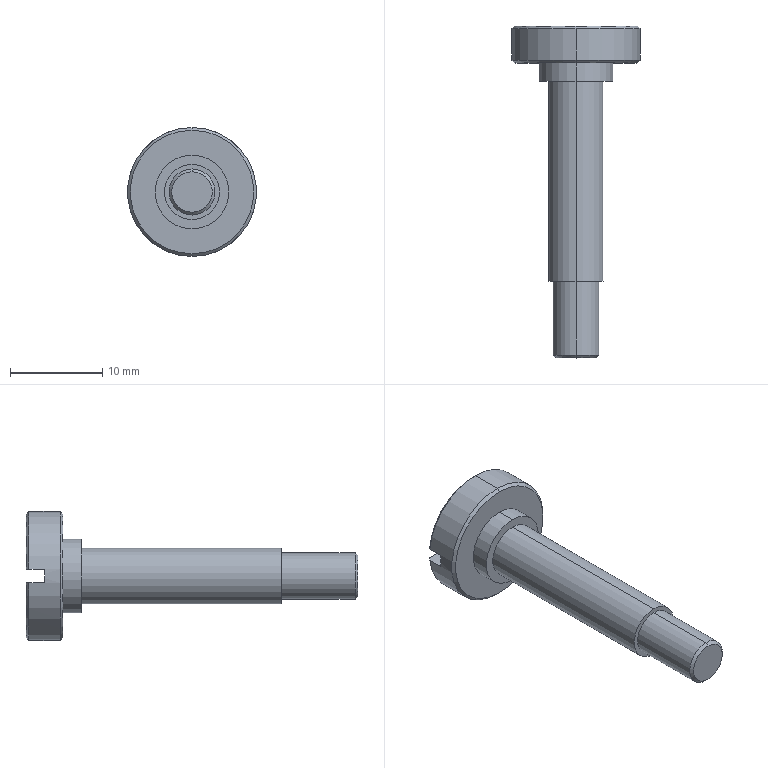Part | SolidWorks | features BaseBody 1 | 1 solid | 24 faces | box 14 x 36 x 14 mm | volume 1446 mm3 | plane 9 | cylinder 8 | cone 7 | commonest cylinder face diameters 5 x2 6 x2 8 x2 14 x2
STEP:
#1=CARTESIAN_POINT('',(0.,36.,-6.7));
#2=VERTEX_POINT('',#1);
#3=CARTESIAN_POINT('',(-6.658,36.,-0.75));
#4=VERTEX_POINT('',#3);
#5=CARTESIAN_POINT('',(0.,36.,0.));
#6=DIRECTION('',(0.,1.,0.));
#7=DIRECTION('',(0.,0.,-1.));
#8=AXIS2_PLACEMENT_3D('',#5,#6,#7);
#9=CIRCLE('',#8,6.7);
#10=EDGE_CURVE('',#2,#4,#9,.T.);
#11=ORIENTED_EDGE('',*,*,#10,.F.);
#12=CARTESIAN_POINT('',(0.,35.7,-7.));
#13=VERTEX_POINT('',#12);
#14=CARTESIAN_POINT('',(0.,35.7,-7.));
#15=DIRECTION('',(0.,-0.7071,-0.7071));
#16=VECTOR('',#15,1000.);
#17=LINE('',#14,#16);
#18=EDGE_CURVE('',#2,#13,#17,.T.);
#19=ORIENTED_EDGE('',*,*,#18,.T.);
#20=CARTESIAN_POINT('',(-6.96,35.7,-0.75));
#21=VERTEX_POINT('',#20);
#22=CARTESIAN_POINT('',(0.,35.7,0.));
#23=DIRECTION('',(0.,-1.,0.));
#24=DIRECTION('',(0.,0.,-1.));
#25=AXIS2_PLACEMENT_3D('',#22,#23,#24);
#26=CIRCLE('',#25,7.);
#27=EDGE_CURVE('',#21,#13,#26,.T.);
#28=ORIENTED_EDGE('',*,*,#27,.F.);
#29=CARTESIAN_POINT('',(-6.658,36.,-0.75));
#30=CARTESIAN_POINT('',(-6.759,35.9,-0.75));
#31=CARTESIAN_POINT('',(-6.859,35.8,-0.75));
#32=CARTESIAN_POINT('',(-6.96,35.7,-0.75));
#33=B_SPLINE_CURVE_WITH_KNOTS('',3,(#29,#30,#31,#32),.UNSPECIFIED.,.F.,.F.,(4,4),(0.03037,0.0308),.UNSPECIFIED.);
#34=EDGE_CURVE('',#4,#21,#33,.T.);
#35=ORIENTED_EDGE('',*,*,#34,.F.);
#36=EDGE_LOOP('',(#11,#19,#28,#35));
#37=FACE_OUTER_BOUND('',#36,.T.);
#38=CARTESIAN_POINT('',(0.,35.7,0.));
#39=DIRECTION('',(0.,-1.,0.));
#40=DIRECTION('',(0.,0.,-1.));
#41=AXIS2_PLACEMENT_3D('',#38,#39,#40);
#42=CONICAL_SURFACE('',#41,7.,0.7854);
#43=ADVANCED_FACE('',(#37),#42,.T.);
#44=CARTESIAN_POINT('',(0.,0.,-2.2));
#45=VERTEX_POINT('',#44);
#46=CARTESIAN_POINT('',(0.,0.,2.2));
#47=VERTEX_POINT('',#46);
#48=CARTESIAN_POINT('',(0.,0.,0.));
#49=DIRECTION('',(0.,-1.,0.));
#50=DIRECTION('',(0.,0.,1.));
#51=AXIS2_PLACEMENT_3D('',#48,#49,#50);
#52=CIRCLE('',#51,2.2);
#53=EDGE_CURVE('',#45,#47,#52,.T.);
#54=ORIENTED_EDGE('',*,*,#53,.F.);
#55=CARTESIAN_POINT('',(0.,0.3,-2.5));
#56=VERTEX_POINT('',#55);
#57=CARTESIAN_POINT('',(0.,0.,-2.2));
#58=DIRECTION('',(0.,0.7071,-0.7071));
#59=VECTOR('',#58,1000.);
#60=LINE('',#57,#59);
#61=EDGE_CURVE('',#45,#56,#60,.T.);
#62=ORIENTED_EDGE('',*,*,#61,.T.);
#63=CARTESIAN_POINT('',(0.,0.3,2.5));
#64=VERTEX_POINT('',#63);
#65=CARTESIAN_POINT('',(0.,0.3,0.));
#66=DIRECTION('',(0.,1.,0.));
#67=DIRECTION('',(0.,0.,1.));
#68=AXIS2_PLACEMENT_3D('',#65,#66,#67);
#69=CIRCLE('',#68,2.5);
#70=EDGE_CURVE('',#64,#56,#69,.T.);
#71=ORIENTED_EDGE('',*,*,#70,.F.);
#72=CARTESIAN_POINT('',(0.,0.,2.2));
#73=DIRECTION('',(0.,0.7071,0.7071));
#74=VECTOR('',#73,1000.);
#75=LINE('',#72,#74);
#76=EDGE_CURVE('',#47,#64,#75,.T.);
#77=ORIENTED_EDGE('',*,*,#76,.F.);
#78=EDGE_LOOP('',(#54,#62,#71,#77));
#79=FACE_OUTER_BOUND('',#78,.T.);
#80=CARTESIAN_POINT('',(0.,0.,0.));
#81=DIRECTION('',(0.,1.,0.));
#82=DIRECTION('',(0.,0.,1.));
#83=AXIS2_PLACEMENT_3D('',#80,#81,#82);
#84=CONICAL_SURFACE('',#83,2.2,0.7854);
#85=ADVANCED_FACE('',(#79),#84,.T.);
#86=CARTESIAN_POINT('',(0.,32.,-6.7));
#87=VERTEX_POINT('',#86);
#88=CARTESIAN_POINT('',(0.,32.,6.7));
#89=VERTEX_POINT('',#88);
#90=CARTESIAN_POINT('',(0.,32.,0.));
#91=DIRECTION('',(0.,-1.,0.));
#92=DIRECTION('',(0.,0.,1.));
#93=AXIS2_PLACEMENT_3D('',#90,#91,#92);
#94=CIRCLE('',#93,6.7);
#95=EDGE_CURVE('',#87,#89,#94,.T.);
#96=ORIENTED_EDGE('',*,*,#95,.F.);
#97=CARTESIAN_POINT('',(0.,32.3,-7.));
#98=VERTEX_POINT('',#97);
#99=CARTESIAN_POINT('',(0.,32.,-6.7));
#100=DIRECTION('',(0.,0.7071,-0.7071));
#101=VECTOR('',#100,1000.);
#102=LINE('',#99,#101);
#103=EDGE_CURVE('',#87,#98,#102,.T.);
#104=ORIENTED_EDGE('',*,*,#103,.T.);
#105=CARTESIAN_POINT('',(0.,32.3,7.));
#106=VERTEX_POINT('',#105);
#107=CARTESIAN_POINT('',(0.,32.3,0.));
#108=DIRECTION('',(0.,1.,0.));
#109=DIRECTION('',(0.,0.,1.));
#110=AXIS2_PLACEMENT_3D('',#107,#108,#109);
#111=CIRCLE('',#110,7.);
#112=EDGE_CURVE('',#106,#98,#111,.T.);
#113=ORIENTED_EDGE('',*,*,#112,.F.);
#114=CARTESIAN_POINT('',(0.,32.,6.7));
#115=DIRECTION('',(0.,0.7071,0.7071));
#116=VECTOR('',#115,1000.);
#117=LINE('',#114,#116);
#118=EDGE_CURVE('',#89,#106,#117,.T.);
#119=ORIENTED_EDGE('',*,*,#118,.F.);
#120=EDGE_LOOP('',(#96,#104,#113,#119));
#121=FACE_OUTER_BOUND('',#120,.T.);
#122=CARTESIAN_POINT('',(0.,32.,0.));
#123=DIRECTION('',(0.,1.,0.));
#124=DIRECTION('',(0.,0.,1.));
#125=AXIS2_PLACEMENT_3D('',#122,#123,#124);
#126=CONICAL_SURFACE('',#125,6.7,0.7854);
#127=ADVANCED_FACE('',(#121),#126,.T.);
#128=CARTESIAN_POINT('',(0.,8.3,-2.5));
#129=VERTEX_POINT('',#128);
#130=CARTESIAN_POINT('',(0.,8.3,2.5));
#131=VERTEX_POINT('',#130);
#132=CARTESIAN_POINT('',(0.,8.3,0.));
#133=DIRECTION('',(0.,-1.,0.));
#134=DIRECTION('',(0.,0.,1.));
#135=AXIS2_PLACEMENT_3D('',#132,#133,#134);
#136=CIRCLE('',#135,2.5);
#137=EDGE_CURVE('',#129,#131,#136,.T.);
#138=ORIENTED_EDGE('',*,*,#137,.T.);
#139=CARTESIAN_POINT('',(0.,51.792,2.5));
#140=DIRECTION('',(0.,-1.,0.));
#141=VECTOR('',#140,1000.);
#142=LINE('',#139,#141);
#143=EDGE_CURVE('',#131,#64,#142,.T.);
#144=ORIENTED_EDGE('',*,*,#143,.T.);
#145=ORIENTED_EDGE('',*,*,#70,.T.);
#146=CARTESIAN_POINT('',(0.,51.792,-2.5));
#147=DIRECTION('',(0.,-1.,0.));
#148=VECTOR('',#147,1000.);
#149=LINE('',#146,#148);
#150=EDGE_CURVE('',#129,#56,#149,.T.);
#151=ORIENTED_EDGE('',*,*,#150,.F.);
#152=EDGE_LOOP('',(#138,#144,#145,#151));
#153=FACE_OUTER_BOUND('',#152,.T.);
#154=CARTESIAN_POINT('',(0.,51.792,0.));
#155=DIRECTION('',(0.,-1.,0.));
#156=DIRECTION('',(0.,0.,-1.));
#157=AXIS2_PLACEMENT_3D('',#154,#155,#156);
#158=CYLINDRICAL_SURFACE('',#157,2.5);
#159=ADVANCED_FACE('',(#153),#158,.T.);
#160=CARTESIAN_POINT('',(0.,30.,-3.));
#161=VERTEX_POINT('',#160);
#162=CARTESIAN_POINT('',(0.,30.,3.));
#163=VERTEX_POINT('',#162);
#164=CARTESIAN_POINT('',(0.,30.,0.));
#165=DIRECTION('',(0.,-1.,0.));
#166=DIRECTION('',(0.,0.,-1.));
#167=AXIS2_PLACEMENT_3D('',#164,#165,#166);
#168=CIRCLE('',#167,3.);
#169=EDGE_CURVE('',#161,#163,#168,.T.);
#170=ORIENTED_EDGE('',*,*,#169,.T.);
#171=CARTESIAN_POINT('',(0.,8.3,3.));
#172=VERTEX_POINT('',#171);
#173=CARTESIAN_POINT('',(0.,0.,3.));
#174=DIRECTION('',(0.,-1.,0.));
#175=VECTOR('',#174,1000.);
#176=LINE('',#173,#175);
#177=EDGE_CURVE('',#163,#172,#176,.T.);
#178=ORIENTED_EDGE('',*,*,#177,.T.);
#179=CARTESIAN_POINT('',(0.,8.3,-3.));
#180=VERTEX_POINT('',#179);
#181=CARTESIAN_POINT('',(0.,8.3,0.));
#182=DIRECTION('',(0.,1.,0.));
#183=DIRECTION('',(0.,0.,1.));
#184=AXIS2_PLACEMENT_3D('',#181,#182,#183);
#185=CIRCLE('',#184,3.);
#186=EDGE_CURVE('',#172,#180,#185,.T.);
#187=ORIENTED_EDGE('',*,*,#186,.T.);
#188=CARTESIAN_POINT('',(0.,0.,-3.));
#189=DIRECTION('',(0.,-1.,0.));
#190=VECTOR('',#189,1000.);
#191=LINE('',#188,#190);
#192=EDGE_CURVE('',#161,#180,#191,.T.);
#193=ORIENTED_EDGE('',*,*,#192,.F.);
#194=EDGE_LOOP('',(#170,#178,#187,#193));
#195=FACE_OUTER_BOUND('',#194,.T.);
#196=CARTESIAN_POINT('',(0.,0.,0.));
#197=DIRECTION('',(0.,-1.,0.));
#198=DIRECTION('',(0.,0.,-1.));
#199=AXIS2_PLACEMENT_3D('',#196,#197,#198);
#200=CYLINDRICAL_SURFACE('',#199,3.);
#201=ADVANCED_FACE('',(#195),#200,.T.);
#202=CARTESIAN_POINT('',(0.,32.,-4.));
#203=VERTEX_POINT('',#202);
#204=CARTESIAN_POINT('',(0.,32.,4.));
#205=VERTEX_POINT('',#204);
#206=CARTESIAN_POINT('',(0.,32.,0.));
#207=DIRECTION('',(0.,-1.,0.));
#208=DIRECTION('',(0.,0.,-1.));
#209=AXIS2_PLACEMENT_3D('',#206,#207,#208);
#210=CIRCLE('',#209,4.);
#211=EDGE_CURVE('',#203,#205,#210,.T.);
#212=ORIENTED_EDGE('',*,*,#211,.T.);
#213=CARTESIAN_POINT('',(0.,30.,4.));
#214=VERTEX_POINT('',#213);
#215=CARTESIAN_POINT('',(0.,0.,4.));
#216=DIRECTION('',(0.,-1.,0.));
#217=VECTOR('',#216,1000.);
#218=LINE('',#215,#217);
#219=EDGE_CURVE('',#205,#214,#218,.T.);
#220=ORIENTED_EDGE('',*,*,#219,.T.);
#221=CARTESIAN_POINT('',(0.,30.,-4.));
#222=VERTEX_POINT('',#221);
#223=CARTESIAN_POINT('',(0.,30.,0.));
#224=DIRECTION('',(0.,-1.,0.));
#225=DIRECTION('',(0.,0.,-1.));
#226=AXIS2_PLACEMENT_3D('',#223,#224,#225);
#227=CIRCLE('',#226,4.);
#228=EDGE_CURVE('',#222,#214,#227,.T.);
#229=ORIENTED_EDGE('',*,*,#228,.F.);
#230=CARTESIAN_POINT('',(0.,0.,-4.));
#231=DIRECTION('',(0.,-1.,0.));
#232=VECTOR('',#231,1000.);
#233=LINE('',#230,#232);
#234=EDGE_CURVE('',#203,#222,#233,.T.);
#235=ORIENTED_EDGE('',*,*,#234,.F.);
#236=EDGE_LOOP('',(#212,#220,#229,#235));
#237=FACE_OUTER_BOUND('',#236,.T.);
#238=CARTESIAN_POINT('',(0.,0.,0.));
#239=DIRECTION('',(0.,-1.,0.));
#240=DIRECTION('',(0.,0.,-1.));
#241=AXIS2_PLACEMENT_3D('',#238,#239,#240);
#242=CYLINDRICAL_SURFACE('',#241,4.);
#243=ADVANCED_FACE('',(#237),#242,.T.);
#244=CARTESIAN_POINT('',(6.96,35.7,0.75));
#245=VERTEX_POINT('',#244);
#246=CARTESIAN_POINT('',(0.,35.7,7.));
#247=VERTEX_POINT('',#246);
#248=CARTESIAN_POINT('',(0.,35.7,0.));
#249=DIRECTION('',(0.,-1.,0.));
#250=DIRECTION('',(0.,0.,-1.));
#251=AXIS2_PLACEMENT_3D('',#248,#249,#250);
#252=CIRCLE('',#251,7.);
#253=EDGE_CURVE('',#245,#247,#252,.T.);
#254=ORIENTED_EDGE('',*,*,#253,.T.);
#255=CARTESIAN_POINT('',(0.,0.,7.));
#256=DIRECTION('',(0.,-1.,0.));
#257=VECTOR('',#256,1000.);
#258=LINE('',#255,#257);
#259=EDGE_CURVE('',#247,#106,#258,.T.);
#260=ORIENTED_EDGE('',*,*,#259,.T.);
#261=ORIENTED_EDGE('',*,*,#112,.T.);
#262=CARTESIAN_POINT('',(0.,0.,-7.));
#263=DIRECTION('',(0.,-1.,0.));
#264=VECTOR('',#263,1000.);
#265=LINE('',#262,#264);
#266=EDGE_CURVE('',#13,#98,#265,.T.);
#267=ORIENTED_EDGE('',*,*,#266,.F.);
#268=CARTESIAN_POINT('',(6.96,35.7,-0.75));
#269=VERTEX_POINT('',#268);
#270=CARTESIAN_POINT('',(0.,35.7,0.));
#271=DIRECTION('',(0.,-1.,0.));
#272=DIRECTION('',(0.,0.,-1.));
#273=AXIS2_PLACEMENT_3D('',#270,#271,#272);
#274=CIRCLE('',#273,7.);
#275=EDGE_CURVE('',#13,#269,#274,.T.);
#276=ORIENTED_EDGE('',*,*,#275,.T.);
#277=CARTESIAN_POINT('',(6.96,34.,-0.75));
#278=VERTEX_POINT('',#277);
#279=CARTESIAN_POINT('',(6.96,0.,-0.75));
#280=DIRECTION('',(0.,-1.,0.));
#281=VECTOR('',#280,1000.);
#282=LINE('',#279,#281);
#283=EDGE_CURVE('',#269,#278,#282,.T.);
#284=ORIENTED_EDGE('',*,*,#283,.T.);
#285=CARTESIAN_POINT('',(6.96,34.,0.75));
#286=VERTEX_POINT('',#285);
#287=CARTESIAN_POINT('',(0.,34.,0.));
#288=DIRECTION('',(0.,-1.,0.));
#289=DIRECTION('',(0.,0.,-1.));
#290=AXIS2_PLACEMENT_3D('',#287,#288,#289);
#291=CIRCLE('',#290,7.);
#292=EDGE_CURVE('',#278,#286,#291,.T.);
#293=ORIENTED_EDGE('',*,*,#292,.T.);
#294=CARTESIAN_POINT('',(6.96,0.,0.75));
#295=DIRECTION('',(0.,1.,0.));
#296=VECTOR('',#295,1000.);
#297=LINE('',#294,#296);
#298=EDGE_CURVE('',#286,#245,#297,.T.);
#299=ORIENTED_EDGE('',*,*,#298,.T.);
#300=EDGE_LOOP('',(#254,#260,#261,#267,#276,#284,#293,#299));
#301=FACE_OUTER_BOUND('',#300,.T.);
#302=CARTESIAN_POINT('',(0.,0.,0.));
#303=DIRECTION('',(0.,-1.,0.));
#304=DIRECTION('',(0.,0.,-1.));
#305=AXIS2_PLACEMENT_3D('',#302,#303,#304);
#306=CYLINDRICAL_SURFACE('',#305,7.);
#307=ADVANCED_FACE('',(#301),#306,.T.);
#308=CARTESIAN_POINT('',(6.658,36.,-0.75));
#309=VERTEX_POINT('',#308);
#310=CARTESIAN_POINT('',(6.96,35.7,-0.75));
#311=CARTESIAN_POINT('',(6.859,35.8,-0.75));
#312=CARTESIAN_POINT('',(6.759,35.9,-0.75));
#313=CARTESIAN_POINT('',(6.658,36.,-0.75));
#314=B_SPLINE_CURVE_WITH_KNOTS('',3,(#310,#311,#312,#313),.UNSPECIFIED.,.F.,.F.,(4,4),(0.0119,0.01232),.UNSPECIFIED.);
#315=EDGE_CURVE('',#269,#309,#314,.T.);
#316=ORIENTED_EDGE('',*,*,#315,.T.);
#317=CARTESIAN_POINT('',(-11.,36.,-0.75));
#318=DIRECTION('',(-1.,0.,0.));
#319=VECTOR('',#318,1000.);
#320=LINE('',#317,#319);
#321=EDGE_CURVE('',#309,#4,#320,.T.);
#322=ORIENTED_EDGE('',*,*,#321,.T.);
#323=ORIENTED_EDGE('',*,*,#34,.T.);
#324=CARTESIAN_POINT('',(-6.96,34.,-0.75));
#325=VERTEX_POINT('',#324);
#326=CARTESIAN_POINT('',(-6.96,0.,-0.75));
#327=DIRECTION('',(0.,1.,0.));
#328=VECTOR('',#327,1000.);
#329=LINE('',#326,#328);
#330=EDGE_CURVE('',#325,#21,#329,.T.);
#331=ORIENTED_EDGE('',*,*,#330,.F.);
#332=CARTESIAN_POINT('',(-11.,34.,-0.75));
#333=DIRECTION('',(-1.,0.,0.));
#334=VECTOR('',#333,1000.);
#335=LINE('',#332,#334);
#336=EDGE_CURVE('',#278,#325,#335,.T.);
#337=ORIENTED_EDGE('',*,*,#336,.F.);
#338=ORIENTED_EDGE('',*,*,#283,.F.);
#339=EDGE_LOOP('',(#316,#322,#323,#331,#337,#338));
#340=FACE_OUTER_BOUND('',#339,.T.);
#341=CARTESIAN_POINT('',(-11.,34.,-0.75));
#342=DIRECTION('',(0.,0.,-1.));
#343=DIRECTION('',(0.,-1.,0.));
#344=AXIS2_PLACEMENT_3D('',#341,#342,#343);
#345=PLANE('',#344);
#346=ADVANCED_FACE('',(#340),#345,.F.);
#347=CARTESIAN_POINT('',(-6.96,35.7,0.75));
#348=VERTEX_POINT('',#347);
#349=CARTESIAN_POINT('',(-6.658,36.,0.75));
#350=VERTEX_POINT('',#349);
#351=CARTESIAN_POINT('',(-6.96,35.7,0.75));
#352=CARTESIAN_POINT('',(-6.859,35.8,0.75));
#353=CARTESIAN_POINT('',(-6.759,35.9,0.75));
#354=CARTESIAN_POINT('',(-6.658,36.,0.75));
#355=B_SPLINE_CURVE_WITH_KNOTS('',3,(#351,#352,#353,#354),.UNSPECIFIED.,.F.,.F.,(4,4),(0.0119,0.01232),.UNSPECIFIED.);
#356=EDGE_CURVE('',#348,#350,#355,.T.);
#357=ORIENTED_EDGE('',*,*,#356,.T.);
#358=CARTESIAN_POINT('',(6.658,36.,0.75));
#359=VERTEX_POINT('',#358);
#360=CARTESIAN_POINT('',(-11.,36.,0.75));
#361=DIRECTION('',(1.,0.,0.));
#362=VECTOR('',#361,1000.);
#363=LINE('',#360,#362);
#364=EDGE_CURVE('',#350,#359,#363,.T.);
#365=ORIENTED_EDGE('',*,*,#364,.T.);
#366=CARTESIAN_POINT('',(6.658,36.,0.75));
#367=CARTESIAN_POINT('',(6.759,35.9,0.75));
#368=CARTESIAN_POINT('',(6.859,35.8,0.75));
#369=CARTESIAN_POINT('',(6.96,35.7,0.75));
#370=B_SPLINE_CURVE_WITH_KNOTS('',3,(#366,#367,#368,#369),.UNSPECIFIED.,.F.,.F.,(4,4),(0.03037,0.0308),.UNSPECIFIED.);
#371=EDGE_CURVE('',#359,#245,#370,.T.);
#372=ORIENTED_EDGE('',*,*,#371,.T.);
#373=ORIENTED_EDGE('',*,*,#298,.F.);
#374=CARTESIAN_POINT('',(-6.96,34.,0.75));
#375=VERTEX_POINT('',#374);
#376=CARTESIAN_POINT('',(-11.,34.,0.75));
#377=DIRECTION('',(1.,0.,0.));
#378=VECTOR('',#377,1000.);
#379=LINE('',#376,#378);
#380=EDGE_CURVE('',#375,#286,#379,.T.);
#381=ORIENTED_EDGE('',*,*,#380,.F.);
#382=CARTESIAN_POINT('',(-6.96,0.,0.75));
#383=DIRECTION('',(0.,-1.,0.));
#384=VECTOR('',#383,1000.);
#385=LINE('',#382,#384);
#386=EDGE_CURVE('',#348,#375,#385,.T.);
#387=ORIENTED_EDGE('',*,*,#386,.F.);
#388=EDGE_LOOP('',(#357,#365,#372,#373,#381,#387));
#389=FACE_OUTER_BOUND('',#388,.T.);
#390=CARTESIAN_POINT('',(-11.,34.,0.75));
#391=DIRECTION('',(0.,0.,1.));
#392=DIRECTION('',(1.,0.,0.));
#393=AXIS2_PLACEMENT_3D('',#390,#391,#392);
#394=PLANE('',#393);
#395=ADVANCED_FACE('',(#389),#394,.F.);
#396=ORIENTED_EDGE('',*,*,#336,.T.);
#397=CARTESIAN_POINT('',(0.,34.,0.));
#398=DIRECTION('',(0.,-1.,0.));
#399=DIRECTION('',(0.,0.,-1.));
#400=AXIS2_PLACEMENT_3D('',#397,#398,#399);
#401=CIRCLE('',#400,7.);
#402=EDGE_CURVE('',#375,#325,#401,.T.);
#403=ORIENTED_EDGE('',*,*,#402,.F.);
#404=ORIENTED_EDGE('',*,*,#380,.T.);
#405=ORIENTED_EDGE('',*,*,#292,.F.);
#406=EDGE_LOOP('',(#396,#403,#404,#405));
#407=FACE_OUTER_BOUND('',#406,.T.);
#408=CARTESIAN_POINT('',(0.,34.,0.));
#409=DIRECTION('',(0.,-1.,0.));
#410=DIRECTION('',(0.,0.,-1.));
#411=AXIS2_PLACEMENT_3D('',#408,#409,#410);
#412=PLANE('',#411);
#413=ADVANCED_FACE('',(#407),#412,.F.);
#414=CARTESIAN_POINT('',(0.,0.,0.));
#415=DIRECTION('',(0.,-1.,0.));
#416=DIRECTION('',(0.,0.,1.));
#417=AXIS2_PLACEMENT_3D('',#414,#415,#416);
#418=CIRCLE('',#417,2.2);
#419=EDGE_CURVE('',#47,#45,#418,.T.);
#420=ORIENTED_EDGE('',*,*,#419,.T.);
#421=ORIENTED_EDGE('',*,*,#53,.T.);
#422=EDGE_LOOP('',(#420,#421));
#423=FACE_OUTER_BOUND('',#422,.T.);
#424=CARTESIAN_POINT('',(-3.,0.,0.));
#425=DIRECTION('',(0.,1.,0.));
#426=DIRECTION('',(1.,0.,0.));
#427=AXIS2_PLACEMENT_3D('',#424,#425,#426);
#428=PLANE('',#427);
#429=ADVANCED_FACE('',(#423),#428,.F.);
#430=ORIENTED_EDGE('',*,*,#137,.F.);
#431=CARTESIAN_POINT('',(0.,8.3,0.));
#432=DIRECTION('',(0.,-1.,0.));
#433=DIRECTION('',(0.,0.,1.));
#434=AXIS2_PLACEMENT_3D('',#431,#432,#433);
#435=CIRCLE('',#434,2.5);
#436=EDGE_CURVE('',#131,#129,#435,.T.);
#437=ORIENTED_EDGE('',*,*,#436,.F.);
#438=EDGE_LOOP('',(#430,#437));
#439=FACE_BOUND('',#438,.T.);
#440=CARTESIAN_POINT('',(0.,8.3,0.));
#441=DIRECTION('',(0.,1.,0.));
#442=DIRECTION('',(0.,0.,1.));
#443=AXIS2_PLACEMENT_3D('',#440,#441,#442);
#444=CIRCLE('',#443,3.);
#445=EDGE_CURVE('',#180,#172,#444,.T.);
#446=ORIENTED_EDGE('',*,*,#445,.F.);
#447=ORIENTED_EDGE('',*,*,#186,.F.);
#448=EDGE_LOOP('',(#446,#447));
#449=FACE_OUTER_BOUND('',#448,.T.);
#450=CARTESIAN_POINT('',(-4.,8.3,0.));
#451=DIRECTION('',(0.,1.,0.));
#452=DIRECTION('',(1.,0.,0.));
#453=AXIS2_PLACEMENT_3D('',#450,#451,#452);
#454=PLANE('',#453);
#455=ADVANCED_FACE('',(#439,#449),#454,.F.);
#456=ORIENTED_EDGE('',*,*,#169,.F.);
#457=CARTESIAN_POINT('',(0.,30.,0.));
#458=DIRECTION('',(0.,-1.,0.));
#459=DIRECTION('',(0.,0.,-1.));
#460=AXIS2_PLACEMENT_3D('',#457,#458,#459);
#461=CIRCLE('',#460,3.);
#462=EDGE_CURVE('',#163,#161,#461,.T.);
#463=ORIENTED_EDGE('',*,*,#462,.F.);
#464=EDGE_LOOP('',(#456,#463));
#465=FACE_BOUND('',#464,.T.);
#466=ORIENTED_EDGE('',*,*,#228,.T.);
#467=CARTESIAN_POINT('',(0.,30.,0.));
#468=DIRECTION('',(0.,-1.,0.));
#469=DIRECTION('',(0.,0.,-1.));
#470=AXIS2_PLACEMENT_3D('',#467,#468,#469);
#471=CIRCLE('',#470,4.);
#472=EDGE_CURVE('',#214,#222,#471,.T.);
#473=ORIENTED_EDGE('',*,*,#472,.T.);
#474=EDGE_LOOP('',(#466,#473));
#475=FACE_OUTER_BOUND('',#474,.T.);
#476=CARTESIAN_POINT('',(-4.,30.,0.));
#477=DIRECTION('',(0.,1.,0.));
#478=DIRECTION('',(1.,0.,0.));
#479=AXIS2_PLACEMENT_3D('',#476,#477,#478);
#480=PLANE('',#479);
#481=ADVANCED_FACE('',(#465,#475),#480,.F.);
#482=ORIENTED_EDGE('',*,*,#211,.F.);
#483=CARTESIAN_POINT('',(0.,32.,0.));
#484=DIRECTION('',(0.,-1.,0.));
#485=DIRECTION('',(0.,0.,-1.));
#486=AXIS2_PLACEMENT_3D('',#483,#484,#485);
#487=CIRCLE('',#486,4.);
#488=EDGE_CURVE('',#205,#203,#487,.T.);
#489=ORIENTED_EDGE('',*,*,#488,.F.);
#490=EDGE_LOOP('',(#482,#489));
#491=FACE_BOUND('',#490,.T.);
#492=CARTESIAN_POINT('',(0.,32.,0.));
#493=DIRECTION('',(0.,-1.,0.));
#494=DIRECTION('',(0.,0.,1.));
#495=AXIS2_PLACEMENT_3D('',#492,#493,#494);
#496=CIRCLE('',#495,6.7);
#497=EDGE_CURVE('',#89,#87,#496,.T.);
#498=ORIENTED_EDGE('',*,*,#497,.T.);
#499=ORIENTED_EDGE('',*,*,#95,.T.);
#500=EDGE_LOOP('',(#498,#499));
#501=FACE_OUTER_BOUND('',#500,.T.);
#502=CARTESIAN_POINT('',(-7.,32.,0.));
#503=DIRECTION('',(0.,1.,0.));
#504=DIRECTION('',(1.,0.,0.));
#505=AXIS2_PLACEMENT_3D('',#502,#503,#504);
#506=PLANE('',#505);
#507=ADVANCED_FACE('',(#491,#501),#506,.F.);
#508=ORIENTED_EDGE('',*,*,#321,.F.);
#509=CARTESIAN_POINT('',(0.,36.,0.));
#510=DIRECTION('',(0.,1.,0.));
#511=DIRECTION('',(0.,0.,-1.));
#512=AXIS2_PLACEMENT_3D('',#509,#510,#511);
#513=CIRCLE('',#512,6.7);
#514=EDGE_CURVE('',#309,#2,#513,.T.);
#515=ORIENTED_EDGE('',*,*,#514,.T.);
#516=ORIENTED_EDGE('',*,*,#10,.T.);
#517=EDGE_LOOP('',(#508,#515,#516));
#518=FACE_OUTER_BOUND('',#517,.T.);
#519=CARTESIAN_POINT('',(0.,36.,0.));
#520=DIRECTION('',(0.,-1.,0.));
#521=DIRECTION('',(0.,0.,-1.));
#522=AXIS2_PLACEMENT_3D('',#519,#520,#521);
#523=PLANE('',#522);
#524=ADVANCED_FACE('',(#518),#523,.F.);
#525=ORIENTED_EDGE('',*,*,#356,.F.);
#526=CARTESIAN_POINT('',(0.,35.7,0.));
#527=DIRECTION('',(0.,-1.,0.));
#528=DIRECTION('',(0.,0.,-1.));
#529=AXIS2_PLACEMENT_3D('',#526,#527,#528);
#530=CIRCLE('',#529,7.);
#531=EDGE_CURVE('',#247,#348,#530,.T.);
#532=ORIENTED_EDGE('',*,*,#531,.F.);
#533=ORIENTED_EDGE('',*,*,#253,.F.);
#534=ORIENTED_EDGE('',*,*,#371,.F.);
#535=CARTESIAN_POINT('',(0.,36.,0.));
#536=DIRECTION('',(0.,1.,0.));
#537=DIRECTION('',(0.,0.,-1.));
#538=AXIS2_PLACEMENT_3D('',#535,#536,#537);
#539=CIRCLE('',#538,6.7);
#540=EDGE_CURVE('',#350,#359,#539,.T.);
#541=ORIENTED_EDGE('',*,*,#540,.F.);
#542=EDGE_LOOP('',(#525,#532,#533,#534,#541));
#543=FACE_OUTER_BOUND('',#542,.T.);
#544=CARTESIAN_POINT('',(0.,35.7,0.));
#545=DIRECTION('',(0.,-1.,0.));
#546=DIRECTION('',(0.,0.,-1.));
#547=AXIS2_PLACEMENT_3D('',#544,#545,#546);
#548=CONICAL_SURFACE('',#547,7.,0.7854);
#549=ADVANCED_FACE('',(#543),#548,.T.);
#550=ORIENTED_EDGE('',*,*,#540,.T.);
#551=ORIENTED_EDGE('',*,*,#364,.F.);
#552=EDGE_LOOP('',(#550,#551));
#553=FACE_OUTER_BOUND('',#552,.T.);
#554=CARTESIAN_POINT('',(0.,36.,0.));
#555=DIRECTION('',(0.,-1.,0.));
#556=DIRECTION('',(0.,0.,-1.));
#557=AXIS2_PLACEMENT_3D('',#554,#555,#556);
#558=PLANE('',#557);
#559=ADVANCED_FACE('',(#553),#558,.F.);
#560=ORIENTED_EDGE('',*,*,#259,.F.);
#561=ORIENTED_EDGE('',*,*,#531,.T.);
#562=ORIENTED_EDGE('',*,*,#386,.T.);
#563=ORIENTED_EDGE('',*,*,#402,.T.);
#564=ORIENTED_EDGE('',*,*,#330,.T.);
#565=ORIENTED_EDGE('',*,*,#27,.T.);
#566=ORIENTED_EDGE('',*,*,#266,.T.);
#567=CARTESIAN_POINT('',(0.,32.3,0.));
#568=DIRECTION('',(0.,1.,0.));
#569=DIRECTION('',(0.,0.,1.));
#570=AXIS2_PLACEMENT_3D('',#567,#568,#569);
#571=CIRCLE('',#570,7.);
#572=EDGE_CURVE('',#98,#106,#571,.T.);
#573=ORIENTED_EDGE('',*,*,#572,.T.);
#574=EDGE_LOOP('',(#560,#561,#562,#563,#564,#565,#566,#573));
#575=FACE_OUTER_BOUND('',#574,.T.);
#576=CARTESIAN_POINT('',(0.,0.,0.));
#577=DIRECTION('',(0.,-1.,0.));
#578=DIRECTION('',(0.,0.,-1.));
#579=AXIS2_PLACEMENT_3D('',#576,#577,#578);
#580=CYLINDRICAL_SURFACE('',#579,7.);
#581=ADVANCED_FACE('',(#575),#580,.T.);
#582=ORIENTED_EDGE('',*,*,#219,.F.);
#583=ORIENTED_EDGE('',*,*,#488,.T.);
#584=ORIENTED_EDGE('',*,*,#234,.T.);
#585=ORIENTED_EDGE('',*,*,#472,.F.);
#586=EDGE_LOOP('',(#582,#583,#584,#585));
#587=FACE_OUTER_BOUND('',#586,.T.);
#588=CARTESIAN_POINT('',(0.,0.,0.));
#589=DIRECTION('',(0.,-1.,0.));
#590=DIRECTION('',(0.,0.,-1.));
#591=AXIS2_PLACEMENT_3D('',#588,#589,#590);
#592=CYLINDRICAL_SURFACE('',#591,4.);
#593=ADVANCED_FACE('',(#587),#592,.T.);
#594=ORIENTED_EDGE('',*,*,#177,.F.);
#595=ORIENTED_EDGE('',*,*,#462,.T.);
#596=ORIENTED_EDGE('',*,*,#192,.T.);
#597=ORIENTED_EDGE('',*,*,#445,.T.);
#598=EDGE_LOOP('',(#594,#595,#596,#597));
#599=FACE_OUTER_BOUND('',#598,.T.);
#600=CARTESIAN_POINT('',(0.,0.,0.));
#601=DIRECTION('',(0.,-1.,0.));
#602=DIRECTION('',(0.,0.,-1.));
#603=AXIS2_PLACEMENT_3D('',#600,#601,#602);
#604=CYLINDRICAL_SURFACE('',#603,3.);
#605=ADVANCED_FACE('',(#599),#604,.T.);
#606=ORIENTED_EDGE('',*,*,#143,.F.);
#607=ORIENTED_EDGE('',*,*,#436,.T.);
#608=ORIENTED_EDGE('',*,*,#150,.T.);
#609=CARTESIAN_POINT('',(0.,0.3,0.));
#610=DIRECTION('',(0.,1.,0.));
#611=DIRECTION('',(0.,0.,1.));
#612=AXIS2_PLACEMENT_3D('',#609,#610,#611);
#613=CIRCLE('',#612,2.5);
#614=EDGE_CURVE('',#56,#64,#613,.T.);
#615=ORIENTED_EDGE('',*,*,#614,.T.);
#616=EDGE_LOOP('',(#606,#607,#608,#615));
#617=FACE_OUTER_BOUND('',#616,.T.);
#618=CARTESIAN_POINT('',(0.,51.792,0.));
#619=DIRECTION('',(0.,-1.,0.));
#620=DIRECTION('',(0.,0.,-1.));
#621=AXIS2_PLACEMENT_3D('',#618,#619,#620);
#622=CYLINDRICAL_SURFACE('',#621,2.5);
#623=ADVANCED_FACE('',(#617),#622,.T.);
#624=ORIENTED_EDGE('',*,*,#103,.F.);
#625=ORIENTED_EDGE('',*,*,#497,.F.);
#626=ORIENTED_EDGE('',*,*,#118,.T.);
#627=ORIENTED_EDGE('',*,*,#572,.F.);
#628=EDGE_LOOP('',(#624,#625,#626,#627));
#629=FACE_OUTER_BOUND('',#628,.T.);
#630=CARTESIAN_POINT('',(0.,32.,0.));
#631=DIRECTION('',(0.,1.,0.));
#632=DIRECTION('',(0.,0.,1.));
#633=AXIS2_PLACEMENT_3D('',#630,#631,#632);
#634=CONICAL_SURFACE('',#633,6.7,0.7854);
#635=ADVANCED_FACE('',(#629),#634,.T.);
#636=ORIENTED_EDGE('',*,*,#61,.F.);
#637=ORIENTED_EDGE('',*,*,#419,.F.);
#638=ORIENTED_EDGE('',*,*,#76,.T.);
#639=ORIENTED_EDGE('',*,*,#614,.F.);
#640=EDGE_LOOP('',(#636,#637,#638,#639));
#641=FACE_OUTER_BOUND('',#640,.T.);
#642=CARTESIAN_POINT('',(0.,0.,0.));
#643=DIRECTION('',(0.,1.,0.));
#644=DIRECTION('',(0.,0.,1.));
#645=AXIS2_PLACEMENT_3D('',#642,#643,#644);
#646=CONICAL_SURFACE('',#645,2.2,0.7854);
#647=ADVANCED_FACE('',(#641),#646,.T.);
#648=ORIENTED_EDGE('',*,*,#18,.F.);
#649=ORIENTED_EDGE('',*,*,#514,.F.);
#650=ORIENTED_EDGE('',*,*,#315,.F.);
#651=ORIENTED_EDGE('',*,*,#275,.F.);
#652=EDGE_LOOP('',(#648,#649,#650,#651));
#653=FACE_OUTER_BOUND('',#652,.T.);
#654=CARTESIAN_POINT('',(0.,35.7,0.));
#655=DIRECTION('',(0.,-1.,0.));
#656=DIRECTION('',(0.,0.,-1.));
#657=AXIS2_PLACEMENT_3D('',#654,#655,#656);
#658=CONICAL_SURFACE('',#657,7.,0.7854);
#659=ADVANCED_FACE('',(#653),#658,.T.);
#660=CLOSED_SHELL('',(#43,#85,#127,#159,#201,#243,#307,#346,#395,#413,#429,#455,#481,#507,#524,#549,#559,#581,#593,#605,#623,#635,#647,#659));
#661=MANIFOLD_SOLID_BREP('',#660);
#662=CARTESIAN_POINT('',(0.,0.,0.));
#663=DIRECTION('',(0.,0.,1.));
#664=DIRECTION('',(1.,0.,0.));
#665=AXIS2_PLACEMENT_3D('',#662,#663,#664);
#666=(LENGTH_UNIT()NAMED_UNIT(*)SI_UNIT(.MILLI.,.METRE.));
#667=UNCERTAINTY_MEASURE_WITH_UNIT(LENGTH_MEASURE(0.00001),#666,'','');
#668=(NAMED_UNIT(*)PLANE_ANGLE_UNIT()SI_UNIT($,.RADIAN.));
#669=(NAMED_UNIT(*)SI_UNIT($,.STERADIAN.)SOLID_ANGLE_UNIT());
#670=(GEOMETRIC_REPRESENTATION_CONTEXT(3)GLOBAL_UNCERTAINTY_ASSIGNED_CONTEXT((#667))GLOBAL_UNIT_ASSIGNED_CONTEXT((#666,#668,#669))REPRESENTATION_CONTEXT('',''));
#671=ADVANCED_BREP_SHAPE_REPRESENTATION('',(#661,#665),#670);